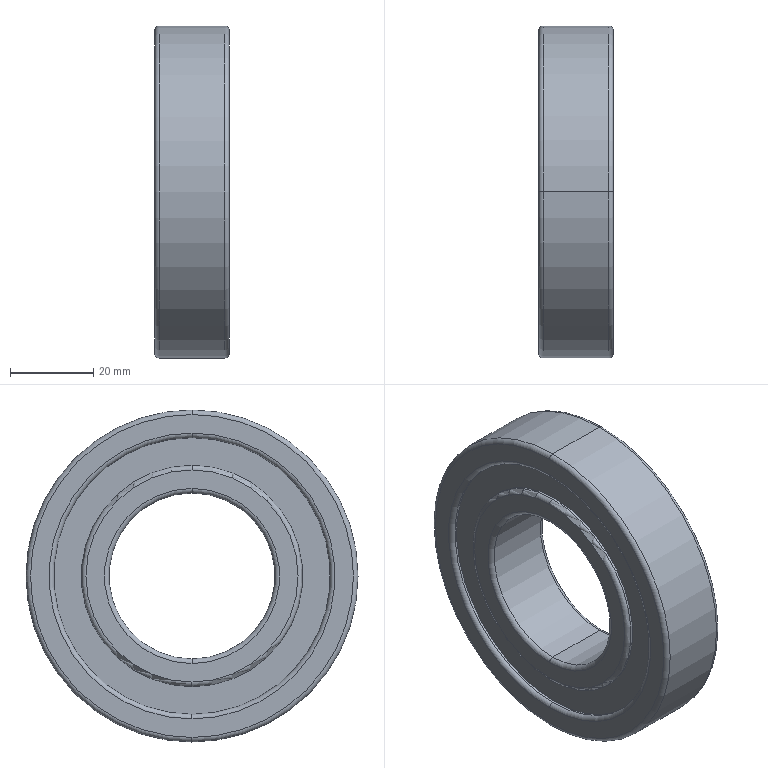Part | SolidWorks | features Revolution 5, CirPattern 2, RefAxis 1, RevCut 1 | 16 solids | 202 faces | box 18 x 80 x 80 mm | volume 53386 mm3 | cylinder 78 | sphere 64 | plane 38 | torus 22 | commonest cylinder face diameters 58 x29 62 x29 53.333 x8 66.667 x8 40 x2 80 x2